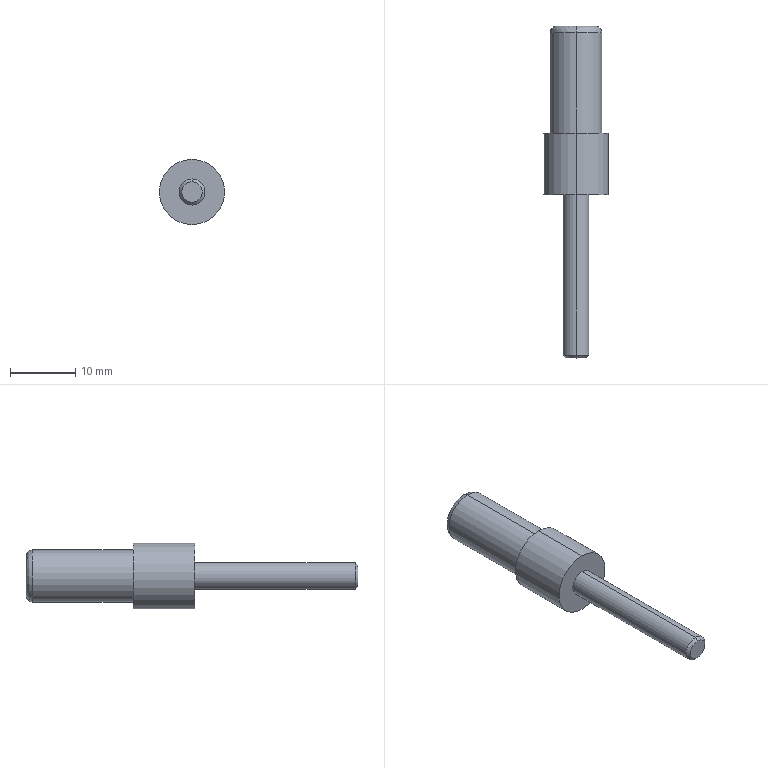Part | STEP file | 0246_Z_006_CLMS4-25-S_1 | 1 solid | 21 faces | box 10 x 50.8 x 10 mm | volume 1847 mm3 | plane 11 | cylinder 6 | spline 2 | cone 2 | commonest cylinder face diameters 4 x2 8 x2 10 x2